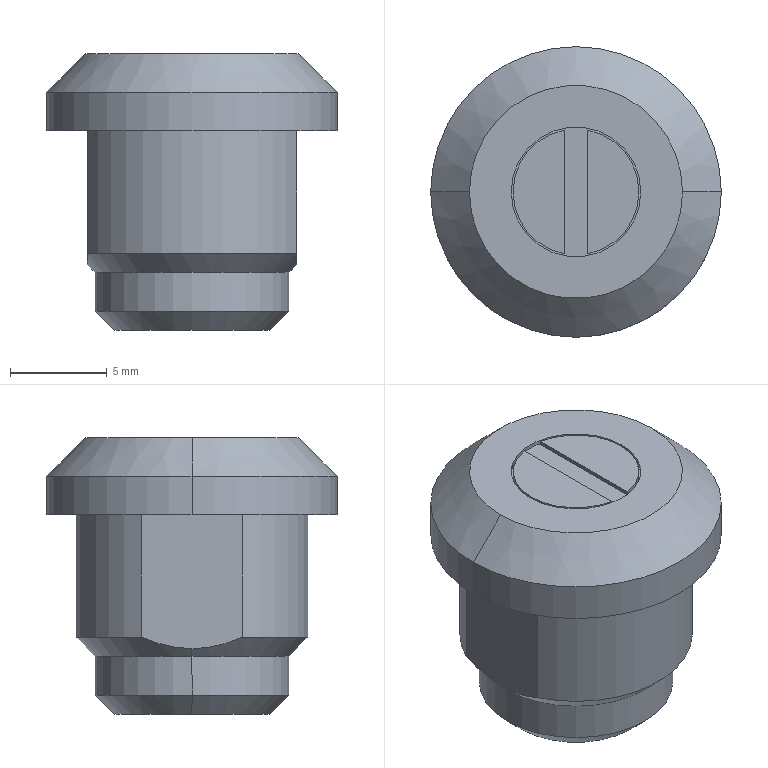Part | SolidWorks | 1 solid | 27 faces | box 15 x 15 x 14.3 mm | volume 1620 mm3 | cylinder 11 | plane 10 | cone 6 | commonest cylinder face diameters 6.5 x3 6.7 x2 10 x2 12 x2 15 x2
STEP:
#1=CARTESIAN_POINT('',(-5.4,-2.615,-6.3));
#2=VERTEX_POINT('',#1);
#3=CARTESIAN_POINT('',(-5.4,-2.615,0.));
#4=VERTEX_POINT('',#3);
#5=CARTESIAN_POINT('',(-5.4,-2.615,-10.3));
#6=DIRECTION('',(0.,0.,1.));
#7=VECTOR('',#6,1000.);
#8=LINE('',#5,#7);
#9=EDGE_CURVE('',#2,#4,#8,.T.);
#10=ORIENTED_EDGE('',*,*,#9,.T.);
#11=CARTESIAN_POINT('',(-5.4,2.615,0.));
#12=VERTEX_POINT('',#11);
#13=CARTESIAN_POINT('',(-5.4,-10.127,0.));
#14=DIRECTION('',(0.,1.,0.));
#15=VECTOR('',#14,1000.);
#16=LINE('',#13,#15);
#17=EDGE_CURVE('',#4,#12,#16,.T.);
#18=ORIENTED_EDGE('',*,*,#17,.T.);
#19=CARTESIAN_POINT('',(-5.4,2.615,-6.3));
#20=VERTEX_POINT('',#19);
#21=CARTESIAN_POINT('',(-5.4,2.615,-10.3));
#22=DIRECTION('',(0.,0.,-1.));
#23=VECTOR('',#22,1000.);
#24=LINE('',#21,#23);
#25=EDGE_CURVE('',#12,#20,#24,.T.);
#26=ORIENTED_EDGE('',*,*,#25,.T.);
#27=CARTESIAN_POINT('',(-5.4,0.,-6.9));
#28=VERTEX_POINT('',#27);
#29=CARTESIAN_POINT('',(-5.4,0.,-6.9));
#30=CARTESIAN_POINT('',(-5.4,0.224,-6.9));
#31=CARTESIAN_POINT('',(-5.4,0.4453,-6.886));
#32=CARTESIAN_POINT('',(-5.4,0.7782,-6.846));
#33=CARTESIAN_POINT('',(-5.4,0.8893,-6.829));
#34=CARTESIAN_POINT('',(-5.4,1.057,-6.798));
#35=CARTESIAN_POINT('',(-5.4,1.141,-6.781));
#36=CARTESIAN_POINT('',(-5.4,1.225,-6.763));
#37=CARTESIAN_POINT('',(-5.4,1.282,-6.75));
#38=CARTESIAN_POINT('',(-5.4,1.312,-6.743));
#39=CARTESIAN_POINT('',(-5.4,1.759,-6.636));
#40=CARTESIAN_POINT('',(-5.4,2.18,-6.49));
#41=CARTESIAN_POINT('',(-5.4,2.615,-6.3));
#42=B_SPLINE_CURVE_WITH_KNOTS('',3,(#29,#30,#31,#32,#33,#34,#35,#36,#37,#38,#39,#40,#41),.UNSPECIFIED.,.F.,.F.,(4,2,2,1,2,2,4),(0.,0.25,0.375,0.4375,0.4688,0.5,1.),.UNSPECIFIED.);
#43=EDGE_CURVE('',#28,#20,#42,.T.);
#44=ORIENTED_EDGE('',*,*,#43,.F.);
#45=CARTESIAN_POINT('',(-5.4,-2.615,-6.3));
#46=CARTESIAN_POINT('',(-5.4,-2.398,-6.395));
#47=CARTESIAN_POINT('',(-5.4,-2.185,-6.478));
#48=CARTESIAN_POINT('',(-5.4,-1.867,-6.587));
#49=CARTESIAN_POINT('',(-5.4,-1.762,-6.621));
#50=CARTESIAN_POINT('',(-5.4,-1.604,-6.667));
#51=CARTESIAN_POINT('',(-5.4,-1.526,-6.689));
#52=CARTESIAN_POINT('',(-5.4,-1.447,-6.71));
#53=CARTESIAN_POINT('',(-5.4,-1.395,-6.723));
#54=CARTESIAN_POINT('',(-5.4,-1.37,-6.729));
#55=CARTESIAN_POINT('',(-5.4,-1.231,-6.763));
#56=CARTESIAN_POINT('',(-5.4,-1.12,-6.786));
#57=CARTESIAN_POINT('',(-5.4,-0.8977,-6.827));
#58=CARTESIAN_POINT('',(-5.4,-0.7891,-6.844));
#59=CARTESIAN_POINT('',(-5.4,-0.4494,-6.886));
#60=CARTESIAN_POINT('',(-5.4,-0.2253,-6.9));
#61=CARTESIAN_POINT('',(-5.4,0.,-6.9));
#62=B_SPLINE_CURVE_WITH_KNOTS('',3,(#45,#46,#47,#48,#49,#50,#51,#52,#53,#54,#55,#56,#57,#58,#59,#60,#61),.UNSPECIFIED.,.F.,.F.,(4,2,2,1,2,2,2,2,4),(0.,0.25,0.375,0.4375,0.4688,0.5,0.625,0.75,1.),.UNSPECIFIED.);
#63=EDGE_CURVE('',#2,#28,#62,.T.);
#64=ORIENTED_EDGE('',*,*,#63,.F.);
#65=EDGE_LOOP('',(#10,#18,#26,#44,#64));
#66=FACE_OUTER_BOUND('',#65,.T.);
#67=CARTESIAN_POINT('',(-5.4,-10.127,25.455));
#68=DIRECTION('',(-1.,0.,0.));
#69=DIRECTION('',(0.,0.,1.));
#70=AXIS2_PLACEMENT_3D('',#67,#68,#69);
#71=PLANE('',#70);
#72=ADVANCED_FACE('',(#66),#71,.T.);
#73=CARTESIAN_POINT('',(5.4,2.615,-6.3));
#74=VERTEX_POINT('',#73);
#75=CARTESIAN_POINT('',(5.4,2.615,0.));
#76=VERTEX_POINT('',#75);
#77=CARTESIAN_POINT('',(5.4,2.615,-10.3));
#78=DIRECTION('',(0.,0.,1.));
#79=VECTOR('',#78,1000.);
#80=LINE('',#77,#79);
#81=EDGE_CURVE('',#74,#76,#80,.T.);
#82=ORIENTED_EDGE('',*,*,#81,.T.);
#83=CARTESIAN_POINT('',(5.4,-2.615,0.));
#84=VERTEX_POINT('',#83);
#85=CARTESIAN_POINT('',(5.4,-10.127,0.));
#86=DIRECTION('',(0.,-1.,0.));
#87=VECTOR('',#86,1000.);
#88=LINE('',#85,#87);
#89=EDGE_CURVE('',#76,#84,#88,.T.);
#90=ORIENTED_EDGE('',*,*,#89,.T.);
#91=CARTESIAN_POINT('',(5.4,-2.615,-6.3));
#92=VERTEX_POINT('',#91);
#93=CARTESIAN_POINT('',(5.4,-2.615,-10.3));
#94=DIRECTION('',(0.,0.,-1.));
#95=VECTOR('',#94,1000.);
#96=LINE('',#93,#95);
#97=EDGE_CURVE('',#84,#92,#96,.T.);
#98=ORIENTED_EDGE('',*,*,#97,.T.);
#99=CARTESIAN_POINT('',(5.4,0.,-6.9));
#100=VERTEX_POINT('',#99);
#101=CARTESIAN_POINT('',(5.4,0.,-6.9));
#102=CARTESIAN_POINT('',(5.4,-0.1126,-6.9));
#103=CARTESIAN_POINT('',(5.4,-0.225,-6.896));
#104=CARTESIAN_POINT('',(5.4,-0.3937,-6.886));
#105=CARTESIAN_POINT('',(5.4,-0.45,-6.882));
#106=CARTESIAN_POINT('',(5.4,-0.5628,-6.871));
#107=CARTESIAN_POINT('',(5.4,-0.6204,-6.865));
#108=CARTESIAN_POINT('',(5.4,-0.7869,-6.844));
#109=CARTESIAN_POINT('',(5.4,-0.8977,-6.827));
#110=CARTESIAN_POINT('',(5.4,-1.064,-6.796));
#111=CARTESIAN_POINT('',(5.4,-1.147,-6.78));
#112=CARTESIAN_POINT('',(5.4,-1.231,-6.762));
#113=CARTESIAN_POINT('',(5.4,-1.287,-6.749));
#114=CARTESIAN_POINT('',(5.4,-1.316,-6.742));
#115=CARTESIAN_POINT('',(5.4,-1.761,-6.635));
#116=CARTESIAN_POINT('',(5.4,-2.181,-6.489));
#117=CARTESIAN_POINT('',(5.4,-2.615,-6.3));
#118=B_SPLINE_CURVE_WITH_KNOTS('',3,(#101,#102,#103,#104,#105,#106,#107,#108,#109,#110,#111,#112,#113,#114,#115,#116,#117),.UNSPECIFIED.,.F.,.F.,(4,2,2,2,2,1,2,2,4),(0.,0.125,0.1875,0.25,0.375,0.4375,0.4687,0.5,1.),.UNSPECIFIED.);
#119=EDGE_CURVE('',#100,#92,#118,.T.);
#120=ORIENTED_EDGE('',*,*,#119,.F.);
#121=CARTESIAN_POINT('',(5.4,2.615,-6.3));
#122=CARTESIAN_POINT('',(5.4,2.397,-6.395));
#123=CARTESIAN_POINT('',(5.4,2.183,-6.479));
#124=CARTESIAN_POINT('',(5.4,1.865,-6.588));
#125=CARTESIAN_POINT('',(5.4,1.759,-6.622));
#126=CARTESIAN_POINT('',(5.4,1.601,-6.668));
#127=CARTESIAN_POINT('',(5.4,1.522,-6.69));
#128=CARTESIAN_POINT('',(5.4,1.443,-6.711));
#129=CARTESIAN_POINT('',(5.4,1.391,-6.724));
#130=CARTESIAN_POINT('',(5.4,1.366,-6.73));
#131=CARTESIAN_POINT('',(5.4,0.8854,-6.846));
#132=CARTESIAN_POINT('',(5.4,0.448,-6.9));
#133=CARTESIAN_POINT('',(5.4,0.,-6.9));
#134=B_SPLINE_CURVE_WITH_KNOTS('',3,(#121,#122,#123,#124,#125,#126,#127,#128,#129,#130,#131,#132,#133),.UNSPECIFIED.,.F.,.F.,(4,2,2,1,2,2,4),(0.,0.25,0.375,0.4375,0.4687,0.5,1.),.UNSPECIFIED.);
#135=EDGE_CURVE('',#74,#100,#134,.T.);
#136=ORIENTED_EDGE('',*,*,#135,.F.);
#137=EDGE_LOOP('',(#82,#90,#98,#120,#136));
#138=FACE_OUTER_BOUND('',#137,.T.);
#139=CARTESIAN_POINT('',(5.4,-10.127,25.455));
#140=DIRECTION('',(1.,0.,0.));
#141=DIRECTION('',(0.,1.,0.));
#142=AXIS2_PLACEMENT_3D('',#139,#140,#141);
#143=PLANE('',#142);
#144=ADVANCED_FACE('',(#138),#143,.T.);
#145=CARTESIAN_POINT('',(-4.,0.,-10.3));
#146=VERTEX_POINT('',#145);
#147=CARTESIAN_POINT('',(-5.,0.,-9.3));
#148=VERTEX_POINT('',#147);
#149=CARTESIAN_POINT('',(-4.,0.,-10.3));
#150=DIRECTION('',(-0.7071,0.,0.7071));
#151=VECTOR('',#150,1000.);
#152=LINE('',#149,#151);
#153=EDGE_CURVE('',#146,#148,#152,.T.);
#154=ORIENTED_EDGE('',*,*,#153,.F.);
#155=CARTESIAN_POINT('',(4.,0.,-10.3));
#156=VERTEX_POINT('',#155);
#157=CARTESIAN_POINT('',(0.,0.,-10.3));
#158=DIRECTION('',(0.,0.,-1.));
#159=DIRECTION('',(-1.,0.,0.));
#160=AXIS2_PLACEMENT_3D('',#157,#158,#159);
#161=CIRCLE('',#160,4.);
#162=EDGE_CURVE('',#156,#146,#161,.T.);
#163=ORIENTED_EDGE('',*,*,#162,.F.);
#164=CARTESIAN_POINT('',(5.,0.,-9.3));
#165=VERTEX_POINT('',#164);
#166=CARTESIAN_POINT('',(4.,0.,-10.3));
#167=DIRECTION('',(0.7071,0.,0.7071));
#168=VECTOR('',#167,1000.);
#169=LINE('',#166,#168);
#170=EDGE_CURVE('',#156,#165,#169,.T.);
#171=ORIENTED_EDGE('',*,*,#170,.T.);
#172=CARTESIAN_POINT('',(0.,0.,-9.3));
#173=DIRECTION('',(0.,0.,1.));
#174=DIRECTION('',(-1.,0.,0.));
#175=AXIS2_PLACEMENT_3D('',#172,#173,#174);
#176=CIRCLE('',#175,5.);
#177=EDGE_CURVE('',#148,#165,#176,.T.);
#178=ORIENTED_EDGE('',*,*,#177,.F.);
#179=EDGE_LOOP('',(#154,#163,#171,#178));
#180=FACE_OUTER_BOUND('',#179,.T.);
#181=CARTESIAN_POINT('',(0.,0.,-10.3));
#182=DIRECTION('',(0.,0.,1.));
#183=DIRECTION('',(1.,0.,0.));
#184=AXIS2_PLACEMENT_3D('',#181,#182,#183);
#185=CONICAL_SURFACE('',#184,4.,0.7854);
#186=ADVANCED_FACE('',(#180),#185,.T.);
#187=ORIENTED_EDGE('',*,*,#162,.T.);
#188=CARTESIAN_POINT('',(0.,0.,-10.3));
#189=DIRECTION('',(0.,0.,-1.));
#190=DIRECTION('',(-1.,0.,0.));
#191=AXIS2_PLACEMENT_3D('',#188,#189,#190);
#192=CIRCLE('',#191,4.);
#193=EDGE_CURVE('',#146,#156,#192,.T.);
#194=ORIENTED_EDGE('',*,*,#193,.T.);
#195=EDGE_LOOP('',(#187,#194));
#196=FACE_OUTER_BOUND('',#195,.T.);
#197=CARTESIAN_POINT('',(0.,0.,-10.3));
#198=DIRECTION('',(0.,0.,-1.));
#199=DIRECTION('',(0.,-1.,0.));
#200=AXIS2_PLACEMENT_3D('',#197,#198,#199);
#201=PLANE('',#200);
#202=ADVANCED_FACE('',(#196),#201,.T.);
#203=CARTESIAN_POINT('',(5.,0.,-7.3));
#204=VERTEX_POINT('',#203);
#205=CARTESIAN_POINT('',(5.,0.,-7.3));
#206=DIRECTION('',(0.,0.,-1.));
#207=VECTOR('',#206,1000.);
#208=LINE('',#205,#207);
#209=EDGE_CURVE('',#204,#165,#208,.T.);
#210=ORIENTED_EDGE('',*,*,#209,.F.);
#211=CARTESIAN_POINT('',(-5.,0.,-7.3));
#212=VERTEX_POINT('',#211);
#213=CARTESIAN_POINT('',(0.,0.,-7.3));
#214=DIRECTION('',(0.,0.,-1.));
#215=DIRECTION('',(-1.,0.,0.));
#216=AXIS2_PLACEMENT_3D('',#213,#214,#215);
#217=CIRCLE('',#216,5.);
#218=EDGE_CURVE('',#204,#212,#217,.T.);
#219=ORIENTED_EDGE('',*,*,#218,.T.);
#220=CARTESIAN_POINT('',(-5.,0.,-7.3));
#221=DIRECTION('',(0.,0.,-1.));
#222=VECTOR('',#221,1000.);
#223=LINE('',#220,#222);
#224=EDGE_CURVE('',#212,#148,#223,.T.);
#225=ORIENTED_EDGE('',*,*,#224,.T.);
#226=ORIENTED_EDGE('',*,*,#177,.T.);
#227=EDGE_LOOP('',(#210,#219,#225,#226));
#228=FACE_OUTER_BOUND('',#227,.T.);
#229=CARTESIAN_POINT('',(0.,0.,-7.3));
#230=DIRECTION('',(0.,0.,-1.));
#231=DIRECTION('',(-1.,0.,0.));
#232=AXIS2_PLACEMENT_3D('',#229,#230,#231);
#233=CYLINDRICAL_SURFACE('',#232,5.);
#234=ADVANCED_FACE('',(#228),#233,.T.);
#235=CARTESIAN_POINT('',(0.6,-3.194,4.));
#236=VERTEX_POINT('',#235);
#237=CARTESIAN_POINT('',(3.25,0.,4.));
#238=VERTEX_POINT('',#237);
#239=CARTESIAN_POINT('',(0.,0.,4.));
#240=DIRECTION('',(0.,0.,1.));
#241=DIRECTION('',(1.,0.,0.));
#242=AXIS2_PLACEMENT_3D('',#239,#240,#241);
#243=CIRCLE('',#242,3.25);
#244=EDGE_CURVE('',#236,#238,#243,.T.);
#245=ORIENTED_EDGE('',*,*,#244,.T.);
#246=CARTESIAN_POINT('',(0.6,3.194,4.));
#247=VERTEX_POINT('',#246);
#248=CARTESIAN_POINT('',(0.,0.,4.));
#249=DIRECTION('',(0.,0.,1.));
#250=DIRECTION('',(1.,0.,0.));
#251=AXIS2_PLACEMENT_3D('',#248,#249,#250);
#252=CIRCLE('',#251,3.25);
#253=EDGE_CURVE('',#238,#247,#252,.T.);
#254=ORIENTED_EDGE('',*,*,#253,.T.);
#255=CARTESIAN_POINT('',(0.6,0.,4.));
#256=DIRECTION('',(0.,-1.,0.));
#257=VECTOR('',#256,1000.);
#258=LINE('',#255,#257);
#259=EDGE_CURVE('',#247,#236,#258,.T.);
#260=ORIENTED_EDGE('',*,*,#259,.T.);
#261=EDGE_LOOP('',(#245,#254,#260));
#262=FACE_OUTER_BOUND('',#261,.T.);
#263=CARTESIAN_POINT('',(0.,0.,4.));
#264=DIRECTION('',(0.,0.,1.));
#265=DIRECTION('',(1.,0.,0.));
#266=AXIS2_PLACEMENT_3D('',#263,#264,#265);
#267=PLANE('',#266);
#268=ADVANCED_FACE('',(#262),#267,.T.);
#269=CARTESIAN_POINT('',(-0.6,3.194,4.));
#270=VERTEX_POINT('',#269);
#271=CARTESIAN_POINT('',(-0.6,-3.194,4.));
#272=VERTEX_POINT('',#271);
#273=CARTESIAN_POINT('',(-0.6,0.,4.));
#274=DIRECTION('',(0.,-1.,0.));
#275=VECTOR('',#274,1000.);
#276=LINE('',#273,#275);
#277=EDGE_CURVE('',#270,#272,#276,.T.);
#278=ORIENTED_EDGE('',*,*,#277,.F.);
#279=CARTESIAN_POINT('',(0.,0.,4.));
#280=DIRECTION('',(0.,0.,1.));
#281=DIRECTION('',(1.,0.,0.));
#282=AXIS2_PLACEMENT_3D('',#279,#280,#281);
#283=CIRCLE('',#282,3.25);
#284=EDGE_CURVE('',#270,#272,#283,.T.);
#285=ORIENTED_EDGE('',*,*,#284,.T.);
#286=EDGE_LOOP('',(#278,#285));
#287=FACE_OUTER_BOUND('',#286,.T.);
#288=CARTESIAN_POINT('',(0.,0.,4.));
#289=DIRECTION('',(0.,0.,1.));
#290=DIRECTION('',(1.,0.,0.));
#291=AXIS2_PLACEMENT_3D('',#288,#289,#290);
#292=PLANE('',#291);
#293=ADVANCED_FACE('',(#287),#292,.T.);
#294=CARTESIAN_POINT('',(0.6,3.194,3.8));
#295=VERTEX_POINT('',#294);
#296=CARTESIAN_POINT('',(0.6,-3.194,3.8));
#297=VERTEX_POINT('',#296);
#298=CARTESIAN_POINT('',(0.6,0.,3.8));
#299=DIRECTION('',(0.,-1.,0.));
#300=VECTOR('',#299,1000.);
#301=LINE('',#298,#300);
#302=EDGE_CURVE('',#295,#297,#301,.T.);
#303=ORIENTED_EDGE('',*,*,#302,.F.);
#304=CARTESIAN_POINT('',(3.25,0.,3.8));
#305=VERTEX_POINT('',#304);
#306=CARTESIAN_POINT('',(0.,0.,3.8));
#307=DIRECTION('',(0.,0.,1.));
#308=DIRECTION('',(1.,0.,0.));
#309=AXIS2_PLACEMENT_3D('',#306,#307,#308);
#310=CIRCLE('',#309,3.25);
#311=EDGE_CURVE('',#305,#295,#310,.T.);
#312=ORIENTED_EDGE('',*,*,#311,.F.);
#313=CARTESIAN_POINT('',(0.,0.,3.8));
#314=DIRECTION('',(0.,0.,1.));
#315=DIRECTION('',(1.,0.,0.));
#316=AXIS2_PLACEMENT_3D('',#313,#314,#315);
#317=CIRCLE('',#316,3.25);
#318=EDGE_CURVE('',#297,#305,#317,.T.);
#319=ORIENTED_EDGE('',*,*,#318,.F.);
#320=EDGE_LOOP('',(#303,#312,#319));
#321=FACE_BOUND('',#320,.T.);
#322=CARTESIAN_POINT('',(-0.6,3.194,3.8));
#323=VERTEX_POINT('',#322);
#324=CARTESIAN_POINT('',(-0.6,-3.194,3.8));
#325=VERTEX_POINT('',#324);
#326=CARTESIAN_POINT('',(0.,0.,3.8));
#327=DIRECTION('',(0.,0.,1.));
#328=DIRECTION('',(1.,0.,0.));
#329=AXIS2_PLACEMENT_3D('',#326,#327,#328);
#330=CIRCLE('',#329,3.25);
#331=EDGE_CURVE('',#323,#325,#330,.T.);
#332=ORIENTED_EDGE('',*,*,#331,.F.);
#333=CARTESIAN_POINT('',(-0.6,0.,3.8));
#334=DIRECTION('',(0.,-1.,0.));
#335=VECTOR('',#334,1000.);
#336=LINE('',#333,#335);
#337=EDGE_CURVE('',#323,#325,#336,.T.);
#338=ORIENTED_EDGE('',*,*,#337,.T.);
#339=EDGE_LOOP('',(#332,#338));
#340=FACE_BOUND('',#339,.T.);
#341=CARTESIAN_POINT('',(3.35,0.,3.8));
#342=VERTEX_POINT('',#341);
#343=CARTESIAN_POINT('',(-3.35,0.,3.8));
#344=VERTEX_POINT('',#343);
#345=CARTESIAN_POINT('',(0.,0.,3.8));
#346=DIRECTION('',(0.,0.,1.));
#347=DIRECTION('',(1.,0.,0.));
#348=AXIS2_PLACEMENT_3D('',#345,#346,#347);
#349=CIRCLE('',#348,3.35);
#350=EDGE_CURVE('',#342,#344,#349,.T.);
#351=ORIENTED_EDGE('',*,*,#350,.T.);
#352=CARTESIAN_POINT('',(0.,0.,3.8));
#353=DIRECTION('',(0.,0.,1.));
#354=DIRECTION('',(1.,0.,0.));
#355=AXIS2_PLACEMENT_3D('',#352,#353,#354);
#356=CIRCLE('',#355,3.35);
#357=EDGE_CURVE('',#344,#342,#356,.T.);
#358=ORIENTED_EDGE('',*,*,#357,.T.);
#359=EDGE_LOOP('',(#351,#358));
#360=FACE_OUTER_BOUND('',#359,.T.);
#361=CARTESIAN_POINT('',(0.,0.,3.8));
#362=DIRECTION('',(0.,0.,1.));
#363=DIRECTION('',(1.,0.,0.));
#364=AXIS2_PLACEMENT_3D('',#361,#362,#363);
#365=PLANE('',#364);
#366=ADVANCED_FACE('',(#321,#340,#360),#365,.T.);
#367=CARTESIAN_POINT('',(-3.35,0.,4.));
#368=VERTEX_POINT('',#367);
#369=CARTESIAN_POINT('',(-3.35,0.,3.8));
#370=DIRECTION('',(0.,0.,1.));
#371=VECTOR('',#370,1000.);
#372=LINE('',#369,#371);
#373=EDGE_CURVE('',#344,#368,#372,.T.);
#374=ORIENTED_EDGE('',*,*,#373,.F.);
#375=ORIENTED_EDGE('',*,*,#350,.F.);
#376=CARTESIAN_POINT('',(3.35,0.,4.));
#377=VERTEX_POINT('',#376);
#378=CARTESIAN_POINT('',(3.35,0.,3.8));
#379=DIRECTION('',(0.,0.,1.));
#380=VECTOR('',#379,1000.);
#381=LINE('',#378,#380);
#382=EDGE_CURVE('',#342,#377,#381,.T.);
#383=ORIENTED_EDGE('',*,*,#382,.T.);
#384=CARTESIAN_POINT('',(0.,0.,4.));
#385=DIRECTION('',(0.,0.,1.));
#386=DIRECTION('',(1.,0.,0.));
#387=AXIS2_PLACEMENT_3D('',#384,#385,#386);
#388=CIRCLE('',#387,3.35);
#389=EDGE_CURVE('',#377,#368,#388,.T.);
#390=ORIENTED_EDGE('',*,*,#389,.T.);
#391=EDGE_LOOP('',(#374,#375,#383,#390));
#392=FACE_OUTER_BOUND('',#391,.T.);
#393=CARTESIAN_POINT('',(0.,0.,3.8));
#394=DIRECTION('',(0.,0.,1.));
#395=DIRECTION('',(1.,0.,0.));
#396=AXIS2_PLACEMENT_3D('',#393,#394,#395);
#397=CYLINDRICAL_SURFACE('',#396,3.35);
#398=ADVANCED_FACE('',(#392),#397,.F.);
#399=ORIENTED_EDGE('',*,*,#277,.T.);
#400=CARTESIAN_POINT('',(-0.6,-3.194,3.8));
#401=DIRECTION('',(0.,0.,1.));
#402=VECTOR('',#401,1000.);
#403=LINE('',#400,#402);
#404=EDGE_CURVE('',#325,#272,#403,.T.);
#405=ORIENTED_EDGE('',*,*,#404,.F.);
#406=ORIENTED_EDGE('',*,*,#337,.F.);
#407=CARTESIAN_POINT('',(-0.6,3.194,3.8));
#408=DIRECTION('',(0.,0.,1.));
#409=VECTOR('',#408,1000.);
#410=LINE('',#407,#409);
#411=EDGE_CURVE('',#323,#270,#410,.T.);
#412=ORIENTED_EDGE('',*,*,#411,.T.);
#413=EDGE_LOOP('',(#399,#405,#406,#412));
#414=FACE_OUTER_BOUND('',#413,.T.);
#415=CARTESIAN_POINT('',(-0.6,0.,3.8));
#416=DIRECTION('',(-1.,0.,0.));
#417=DIRECTION('',(0.,0.,1.));
#418=AXIS2_PLACEMENT_3D('',#415,#416,#417);
#419=PLANE('',#418);
#420=ADVANCED_FACE('',(#414),#419,.F.);
#421=CARTESIAN_POINT('',(3.25,0.,3.8));
#422=DIRECTION('',(0.,0.,1.));
#423=VECTOR('',#422,1000.);
#424=LINE('',#421,#423);
#425=EDGE_CURVE('',#305,#238,#424,.T.);
#426=ORIENTED_EDGE('',*,*,#425,.F.);
#427=ORIENTED_EDGE('',*,*,#311,.T.);
#428=CARTESIAN_POINT('',(0.6,3.194,3.8));
#429=DIRECTION('',(0.,0.,1.));
#430=VECTOR('',#429,1000.);
#431=LINE('',#428,#430);
#432=EDGE_CURVE('',#295,#247,#431,.T.);
#433=ORIENTED_EDGE('',*,*,#432,.T.);
#434=ORIENTED_EDGE('',*,*,#253,.F.);
#435=EDGE_LOOP('',(#426,#427,#433,#434));
#436=FACE_OUTER_BOUND('',#435,.T.);
#437=CARTESIAN_POINT('',(0.,0.,3.8));
#438=DIRECTION('',(0.,0.,1.));
#439=DIRECTION('',(1.,0.,0.));
#440=AXIS2_PLACEMENT_3D('',#437,#438,#439);
#441=CYLINDRICAL_SURFACE('',#440,3.25);
#442=ADVANCED_FACE('',(#436),#441,.T.);
#443=ORIENTED_EDGE('',*,*,#284,.F.);
#444=ORIENTED_EDGE('',*,*,#411,.F.);
#445=ORIENTED_EDGE('',*,*,#331,.T.);
#446=ORIENTED_EDGE('',*,*,#404,.T.);
#447=EDGE_LOOP('',(#443,#444,#445,#446));
#448=FACE_OUTER_BOUND('',#447,.T.);
#449=CARTESIAN_POINT('',(0.,0.,3.8));
#450=DIRECTION('',(0.,0.,1.));
#451=DIRECTION('',(1.,0.,0.));
#452=AXIS2_PLACEMENT_3D('',#449,#450,#451);
#453=CYLINDRICAL_SURFACE('',#452,3.25);
#454=ADVANCED_FACE('',(#448),#453,.T.);
#455=ORIENTED_EDGE('',*,*,#259,.F.);
#456=ORIENTED_EDGE('',*,*,#432,.F.);
#457=ORIENTED_EDGE('',*,*,#302,.T.);
#458=CARTESIAN_POINT('',(0.6,-3.194,3.8));
#459=DIRECTION('',(0.,0.,1.));
#460=VECTOR('',#459,1000.);
#461=LINE('',#458,#460);
#462=EDGE_CURVE('',#297,#236,#461,.T.);
#463=ORIENTED_EDGE('',*,*,#462,.T.);
#464=EDGE_LOOP('',(#455,#456,#457,#463));
#465=FACE_OUTER_BOUND('',#464,.T.);
#466=CARTESIAN_POINT('',(0.6,0.,3.8));
#467=DIRECTION('',(-1.,0.,0.));
#468=DIRECTION('',(0.,0.,1.));
#469=AXIS2_PLACEMENT_3D('',#466,#467,#468);
#470=PLANE('',#469);
#471=ADVANCED_FACE('',(#465),#470,.T.);
#472=CARTESIAN_POINT('',(5.5,0.,4.));
#473=VERTEX_POINT('',#472);
#474=CARTESIAN_POINT('',(7.5,0.,2.));
#475=VERTEX_POINT('',#474);
#476=CARTESIAN_POINT('',(5.5,0.,4.));
#477=DIRECTION('',(0.7071,0.,-0.7071));
#478=VECTOR('',#477,1000.);
#479=LINE('',#476,#478);
#480=EDGE_CURVE('',#473,#475,#479,.T.);
#481=ORIENTED_EDGE('',*,*,#480,.F.);
#482=CARTESIAN_POINT('',(-5.5,0.,4.));
#483=VERTEX_POINT('',#482);
#484=CARTESIAN_POINT('',(0.,0.,4.));
#485=DIRECTION('',(0.,0.,1.));
#486=DIRECTION('',(1.,0.,0.));
#487=AXIS2_PLACEMENT_3D('',#484,#485,#486);
#488=CIRCLE('',#487,5.5);
#489=EDGE_CURVE('',#483,#473,#488,.T.);
#490=ORIENTED_EDGE('',*,*,#489,.F.);
#491=CARTESIAN_POINT('',(-7.5,0.,2.));
#492=VERTEX_POINT('',#491);
#493=CARTESIAN_POINT('',(-5.5,0.,4.));
#494=DIRECTION('',(-0.7071,0.,-0.7071));
#495=VECTOR('',#494,1000.);
#496=LINE('',#493,#495);
#497=EDGE_CURVE('',#483,#492,#496,.T.);
#498=ORIENTED_EDGE('',*,*,#497,.T.);
#499=CARTESIAN_POINT('',(0.,0.,2.));
#500=DIRECTION('',(0.,0.,-1.));
#501=DIRECTION('',(1.,0.,0.));
#502=AXIS2_PLACEMENT_3D('',#499,#500,#501);
#503=CIRCLE('',#502,7.5);
#504=EDGE_CURVE('',#475,#492,#503,.T.);
#505=ORIENTED_EDGE('',*,*,#504,.F.);
#506=EDGE_LOOP('',(#481,#490,#498,#505));
#507=FACE_OUTER_BOUND('',#506,.T.);
#508=CARTESIAN_POINT('',(0.,0.,4.));
#509=DIRECTION('',(0.,0.,-1.));
#510=DIRECTION('',(-1.,0.,0.));
#511=AXIS2_PLACEMENT_3D('',#508,#509,#510);
#512=CONICAL_SURFACE('',#511,5.5,0.7854);
#513=ADVANCED_FACE('',(#507),#512,.T.);
#514=CARTESIAN_POINT('',(0.,0.,0.));
#515=DIRECTION('',(0.,0.,-1.));
#516=DIRECTION('',(-1.,0.,0.));
#517=AXIS2_PLACEMENT_3D('',#514,#515,#516);
#518=CIRCLE('',#517,6.);
#519=EDGE_CURVE('',#12,#76,#518,.T.);
#520=ORIENTED_EDGE('',*,*,#519,.F.);
#521=ORIENTED_EDGE('',*,*,#17,.F.);
#522=CARTESIAN_POINT('',(0.,0.,0.));
#523=DIRECTION('',(0.,0.,-1.));
#524=DIRECTION('',(-1.,0.,0.));
#525=AXIS2_PLACEMENT_3D('',#522,#523,#524);
#526=CIRCLE('',#525,6.);
#527=EDGE_CURVE('',#84,#4,#526,.T.);
#528=ORIENTED_EDGE('',*,*,#527,.F.);
#529=ORIENTED_EDGE('',*,*,#89,.F.);
#530=EDGE_LOOP('',(#520,#521,#528,#529));
#531=FACE_BOUND('',#530,.T.);
#532=CARTESIAN_POINT('',(-7.5,0.,0.));
#533=VERTEX_POINT('',#532);
#534=CARTESIAN_POINT('',(7.5,0.,0.));
#535=VERTEX_POINT('',#534);
#536=CARTESIAN_POINT('',(0.,0.,0.));
#537=DIRECTION('',(0.,0.,1.));
#538=DIRECTION('',(1.,0.,0.));
#539=AXIS2_PLACEMENT_3D('',#536,#537,#538);
#540=CIRCLE('',#539,7.5);
#541=EDGE_CURVE('',#533,#535,#540,.T.);
#542=ORIENTED_EDGE('',*,*,#541,.F.);
#543=CARTESIAN_POINT('',(0.,0.,0.));
#544=DIRECTION('',(0.,0.,1.));
#545=DIRECTION('',(1.,0.,0.));
#546=AXIS2_PLACEMENT_3D('',#543,#544,#545);
#547=CIRCLE('',#546,7.5);
#548=EDGE_CURVE('',#535,#533,#547,.T.);
#549=ORIENTED_EDGE('',*,*,#548,.F.);
#550=EDGE_LOOP('',(#542,#549));
#551=FACE_OUTER_BOUND('',#550,.T.);
#552=CARTESIAN_POINT('',(0.,0.,0.));
#553=DIRECTION('',(0.,0.,1.));
#554=DIRECTION('',(1.,0.,0.));
#555=AXIS2_PLACEMENT_3D('',#552,#553,#554);
#556=PLANE('',#555);
#557=ADVANCED_FACE('',(#531,#551),#556,.F.);
#558=ORIENTED_EDGE('',*,*,#389,.F.);
#559=CARTESIAN_POINT('',(0.,0.,4.));
#560=DIRECTION('',(0.,0.,1.));
#561=DIRECTION('',(1.,0.,0.));
#562=AXIS2_PLACEMENT_3D('',#559,#560,#561);
#563=CIRCLE('',#562,3.35);
#564=EDGE_CURVE('',#368,#377,#563,.T.);
#565=ORIENTED_EDGE('',*,*,#564,.F.);
#566=EDGE_LOOP('',(#558,#565));
#567=FACE_BOUND('',#566,.T.);
#568=ORIENTED_EDGE('',*,*,#489,.T.);
#569=CARTESIAN_POINT('',(0.,0.,4.));
#570=DIRECTION('',(0.,0.,1.));
#571=DIRECTION('',(1.,0.,0.));
#572=AXIS2_PLACEMENT_3D('',#569,#570,#571);
#573=CIRCLE('',#572,5.5);
#574=EDGE_CURVE('',#473,#483,#573,.T.);
#575=ORIENTED_EDGE('',*,*,#574,.T.);
#576=EDGE_LOOP('',(#568,#575));
#577=FACE_OUTER_BOUND('',#576,.T.);
#578=CARTESIAN_POINT('',(0.,0.,4.));
#579=DIRECTION('',(0.,0.,1.));
#580=DIRECTION('',(1.,0.,0.));
#581=AXIS2_PLACEMENT_3D('',#578,#579,#580);
#582=PLANE('',#581);
#583=ADVANCED_FACE('',(#567,#577),#582,.T.);
#584=CARTESIAN_POINT('',(7.5,0.,4.));
#585=DIRECTION('',(0.,0.,-1.));
#586=VECTOR('',#585,1000.);
#587=LINE('',#584,#586);
#588=EDGE_CURVE('',#475,#535,#587,.T.);
#589=ORIENTED_EDGE('',*,*,#588,.F.);
#590=ORIENTED_EDGE('',*,*,#504,.T.);
#591=CARTESIAN_POINT('',(-7.5,0.,4.));
#592=DIRECTION('',(0.,0.,-1.));
#593=VECTOR('',#592,1000.);
#594=LINE('',#591,#593);
#595=EDGE_CURVE('',#492,#533,#594,.T.);
#596=ORIENTED_EDGE('',*,*,#595,.T.);
#597=ORIENTED_EDGE('',*,*,#541,.T.);
#598=EDGE_LOOP('',(#589,#590,#596,#597));
#599=FACE_OUTER_BOUND('',#598,.T.);
#600=CARTESIAN_POINT('',(0.,0.,4.));
#601=DIRECTION('',(0.,0.,-1.));
#602=DIRECTION('',(-1.,0.,0.));
#603=AXIS2_PLACEMENT_3D('',#600,#601,#602);
#604=CYLINDRICAL_SURFACE('',#603,7.5);
#605=ADVANCED_FACE('',(#599),#604,.T.);
#606=CARTESIAN_POINT('',(-5.,0.,-7.3));
#607=DIRECTION('',(-0.7071,0.,0.7071));
#608=VECTOR('',#607,1000.);
#609=LINE('',#606,#608);
#610=EDGE_CURVE('',#212,#28,#609,.T.);
#611=ORIENTED_EDGE('',*,*,#610,.F.);
#612=ORIENTED_EDGE('',*,*,#218,.F.);
#613=CARTESIAN_POINT('',(5.,0.,-7.3));
#614=DIRECTION('',(0.7071,0.,0.7071));
#615=VECTOR('',#614,1000.);
#616=LINE('',#613,#615);
#617=EDGE_CURVE('',#204,#100,#616,.T.);
#618=ORIENTED_EDGE('',*,*,#617,.T.);
#619=ORIENTED_EDGE('',*,*,#119,.T.);
#620=CARTESIAN_POINT('',(0.,0.,-6.3));
#621=DIRECTION('',(0.,0.,1.));
#622=DIRECTION('',(-1.,0.,0.));
#623=AXIS2_PLACEMENT_3D('',#620,#621,#622);
#624=CIRCLE('',#623,6.);
#625=EDGE_CURVE('',#2,#92,#624,.T.);
#626=ORIENTED_EDGE('',*,*,#625,.F.);
#627=ORIENTED_EDGE('',*,*,#63,.T.);
#628=EDGE_LOOP('',(#611,#612,#618,#619,#626,#627));
#629=FACE_OUTER_BOUND('',#628,.T.);
#630=CARTESIAN_POINT('',(0.,0.,-7.3));
#631=DIRECTION('',(0.,0.,1.));
#632=DIRECTION('',(1.,0.,0.));
#633=AXIS2_PLACEMENT_3D('',#630,#631,#632);
#634=CONICAL_SURFACE('',#633,5.,0.7854);
#635=ADVANCED_FACE('',(#629),#634,.T.);
#636=ORIENTED_EDGE('',*,*,#25,.F.);
#637=ORIENTED_EDGE('',*,*,#519,.T.);
#638=ORIENTED_EDGE('',*,*,#81,.F.);
#639=CARTESIAN_POINT('',(0.,0.,-6.3));
#640=DIRECTION('',(0.,0.,1.));
#641=DIRECTION('',(-1.,0.,0.));
#642=AXIS2_PLACEMENT_3D('',#639,#640,#641);
#643=CIRCLE('',#642,6.);
#644=EDGE_CURVE('',#74,#20,#643,.T.);
#645=ORIENTED_EDGE('',*,*,#644,.T.);
#646=EDGE_LOOP('',(#636,#637,#638,#645));
#647=FACE_OUTER_BOUND('',#646,.T.);
#648=CARTESIAN_POINT('',(0.,0.,-10.3));
#649=DIRECTION('',(0.,0.,1.));
#650=DIRECTION('',(1.,0.,0.));
#651=AXIS2_PLACEMENT_3D('',#648,#649,#650);
#652=CYLINDRICAL_SURFACE('',#651,6.);
#653=ADVANCED_FACE('',(#647),#652,.T.);
#654=ORIENTED_EDGE('',*,*,#9,.F.);
#655=ORIENTED_EDGE('',*,*,#625,.T.);
#656=ORIENTED_EDGE('',*,*,#97,.F.);
#657=ORIENTED_EDGE('',*,*,#527,.T.);
#658=EDGE_LOOP('',(#654,#655,#656,#657));
#659=FACE_OUTER_BOUND('',#658,.T.);
#660=CARTESIAN_POINT('',(0.,0.,-10.3));
#661=DIRECTION('',(0.,0.,1.));
#662=DIRECTION('',(1.,0.,0.));
#663=AXIS2_PLACEMENT_3D('',#660,#661,#662);
#664=CYLINDRICAL_SURFACE('',#663,6.);
#665=ADVANCED_FACE('',(#659),#664,.T.);
#666=CARTESIAN_POINT('',(0.,0.,-7.3));
#667=DIRECTION('',(0.,0.,-1.));
#668=DIRECTION('',(-1.,0.,0.));
#669=AXIS2_PLACEMENT_3D('',#666,#667,#668);
#670=CIRCLE('',#669,5.);
#671=EDGE_CURVE('',#212,#204,#670,.T.);
#672=ORIENTED_EDGE('',*,*,#671,.F.);
#673=ORIENTED_EDGE('',*,*,#610,.T.);
#674=ORIENTED_EDGE('',*,*,#43,.T.);
#675=ORIENTED_EDGE('',*,*,#644,.F.);
#676=ORIENTED_EDGE('',*,*,#135,.T.);
#677=ORIENTED_EDGE('',*,*,#617,.F.);
#678=EDGE_LOOP('',(#672,#673,#674,#675,#676,#677));
#679=FACE_OUTER_BOUND('',#678,.T.);
#680=CARTESIAN_POINT('',(0.,0.,-7.3));
#681=DIRECTION('',(0.,0.,1.));
#682=DIRECTION('',(1.,0.,0.));
#683=AXIS2_PLACEMENT_3D('',#680,#681,#682);
#684=CONICAL_SURFACE('',#683,5.,0.7854);
#685=ADVANCED_FACE('',(#679),#684,.T.);
#686=CARTESIAN_POINT('',(0.,0.,2.));
#687=DIRECTION('',(0.,0.,-1.));
#688=DIRECTION('',(1.,0.,0.));
#689=AXIS2_PLACEMENT_3D('',#686,#687,#688);
#690=CIRCLE('',#689,7.5);
#691=EDGE_CURVE('',#492,#475,#690,.T.);
#692=ORIENTED_EDGE('',*,*,#691,.T.);
#693=ORIENTED_EDGE('',*,*,#588,.T.);
#694=ORIENTED_EDGE('',*,*,#548,.T.);
#695=ORIENTED_EDGE('',*,*,#595,.F.);
#696=EDGE_LOOP('',(#692,#693,#694,#695));
#697=FACE_OUTER_BOUND('',#696,.T.);
#698=CARTESIAN_POINT('',(0.,0.,4.));
#699=DIRECTION('',(0.,0.,-1.));
#700=DIRECTION('',(-1.,0.,0.));
#701=AXIS2_PLACEMENT_3D('',#698,#699,#700);
#702=CYLINDRICAL_SURFACE('',#701,7.5);
#703=ADVANCED_FACE('',(#697),#702,.T.);
#704=ORIENTED_EDGE('',*,*,#574,.F.);
#705=ORIENTED_EDGE('',*,*,#480,.T.);
#706=ORIENTED_EDGE('',*,*,#691,.F.);
#707=ORIENTED_EDGE('',*,*,#497,.F.);
#708=EDGE_LOOP('',(#704,#705,#706,#707));
#709=FACE_OUTER_BOUND('',#708,.T.);
#710=CARTESIAN_POINT('',(0.,0.,4.));
#711=DIRECTION('',(0.,0.,-1.));
#712=DIRECTION('',(-1.,0.,0.));
#713=AXIS2_PLACEMENT_3D('',#710,#711,#712);
#714=CONICAL_SURFACE('',#713,5.5,0.7854);
#715=ADVANCED_FACE('',(#709),#714,.T.);
#716=ORIENTED_EDGE('',*,*,#318,.T.);
#717=ORIENTED_EDGE('',*,*,#425,.T.);
#718=ORIENTED_EDGE('',*,*,#244,.F.);
#719=ORIENTED_EDGE('',*,*,#462,.F.);
#720=EDGE_LOOP('',(#716,#717,#718,#719));
#721=FACE_OUTER_BOUND('',#720,.T.);
#722=CARTESIAN_POINT('',(0.,0.,3.8));
#723=DIRECTION('',(0.,0.,1.));
#724=DIRECTION('',(1.,0.,0.));
#725=AXIS2_PLACEMENT_3D('',#722,#723,#724);
#726=CYLINDRICAL_SURFACE('',#725,3.25);
#727=ADVANCED_FACE('',(#721),#726,.T.);
#728=ORIENTED_EDGE('',*,*,#357,.F.);
#729=ORIENTED_EDGE('',*,*,#373,.T.);
#730=ORIENTED_EDGE('',*,*,#564,.T.);
#731=ORIENTED_EDGE('',*,*,#382,.F.);
#732=EDGE_LOOP('',(#728,#729,#730,#731));
#733=FACE_OUTER_BOUND('',#732,.T.);
#734=CARTESIAN_POINT('',(0.,0.,3.8));
#735=DIRECTION('',(0.,0.,1.));
#736=DIRECTION('',(1.,0.,0.));
#737=AXIS2_PLACEMENT_3D('',#734,#735,#736);
#738=CYLINDRICAL_SURFACE('',#737,3.35);
#739=ADVANCED_FACE('',(#733),#738,.F.);
#740=ORIENTED_EDGE('',*,*,#671,.T.);
#741=ORIENTED_EDGE('',*,*,#209,.T.);
#742=CARTESIAN_POINT('',(0.,0.,-9.3));
#743=DIRECTION('',(0.,0.,1.));
#744=DIRECTION('',(-1.,0.,0.));
#745=AXIS2_PLACEMENT_3D('',#742,#743,#744);
#746=CIRCLE('',#745,5.);
#747=EDGE_CURVE('',#165,#148,#746,.T.);
#748=ORIENTED_EDGE('',*,*,#747,.T.);
#749=ORIENTED_EDGE('',*,*,#224,.F.);
#750=EDGE_LOOP('',(#740,#741,#748,#749));
#751=FACE_OUTER_BOUND('',#750,.T.);
#752=CARTESIAN_POINT('',(0.,0.,-7.3));
#753=DIRECTION('',(0.,0.,-1.));
#754=DIRECTION('',(-1.,0.,0.));
#755=AXIS2_PLACEMENT_3D('',#752,#753,#754);
#756=CYLINDRICAL_SURFACE('',#755,5.);
#757=ADVANCED_FACE('',(#751),#756,.T.);
#758=ORIENTED_EDGE('',*,*,#193,.F.);
#759=ORIENTED_EDGE('',*,*,#153,.T.);
#760=ORIENTED_EDGE('',*,*,#747,.F.);
#761=ORIENTED_EDGE('',*,*,#170,.F.);
#762=EDGE_LOOP('',(#758,#759,#760,#761));
#763=FACE_OUTER_BOUND('',#762,.T.);
#764=CARTESIAN_POINT('',(0.,0.,-10.3));
#765=DIRECTION('',(0.,0.,1.));
#766=DIRECTION('',(1.,0.,0.));
#767=AXIS2_PLACEMENT_3D('',#764,#765,#766);
#768=CONICAL_SURFACE('',#767,4.,0.7854);
#769=ADVANCED_FACE('',(#763),#768,.T.);
#770=CLOSED_SHELL('',(#72,#144,#186,#202,#234,#268,#293,#366,#398,#420,#442,#454,#471,#513,#557,#583,#605,#635,#653,#665,#685,#703,#715,#727,#739,#757,#769));
#771=MANIFOLD_SOLID_BREP('',#770);
#772=CARTESIAN_POINT('',(0.,0.,0.));
#773=DIRECTION('',(0.,0.,1.));
#774=DIRECTION('',(1.,0.,0.));
#775=AXIS2_PLACEMENT_3D('',#772,#773,#774);
#776=(LENGTH_UNIT()NAMED_UNIT(*)SI_UNIT(.MILLI.,.METRE.));
#777=UNCERTAINTY_MEASURE_WITH_UNIT(LENGTH_MEASURE(0.00001),#776,'','');
#778=(NAMED_UNIT(*)PLANE_ANGLE_UNIT()SI_UNIT($,.RADIAN.));
#779=(NAMED_UNIT(*)SI_UNIT($,.STERADIAN.)SOLID_ANGLE_UNIT());
#780=(GEOMETRIC_REPRESENTATION_CONTEXT(3)GLOBAL_UNCERTAINTY_ASSIGNED_CONTEXT((#777))GLOBAL_UNIT_ASSIGNED_CONTEXT((#776,#778,#779))REPRESENTATION_CONTEXT('',''));
#781=ADVANCED_BREP_SHAPE_REPRESENTATION('',(#771,#775),#780);